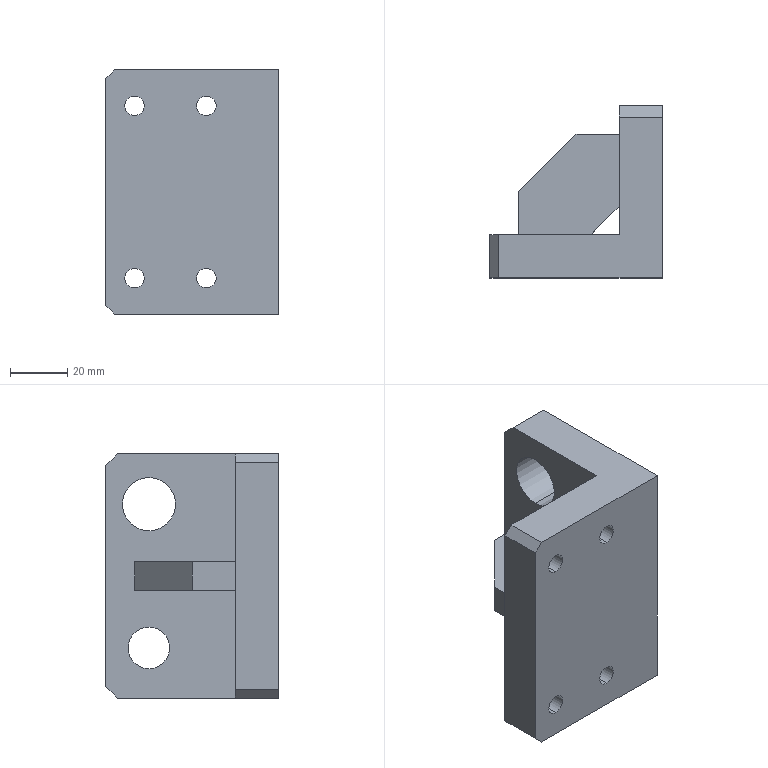Part | STEP file | YCD14007A-08.02.07-Buffer Limit Seat-A3 | 1 solid | 30 faces | box 60 x 60 x 85 mm | volume 134562 mm3 | plane 18 | cylinder 12 | commonest cylinder face diameters 6.8 x8 14.5 x2 18.5 x2